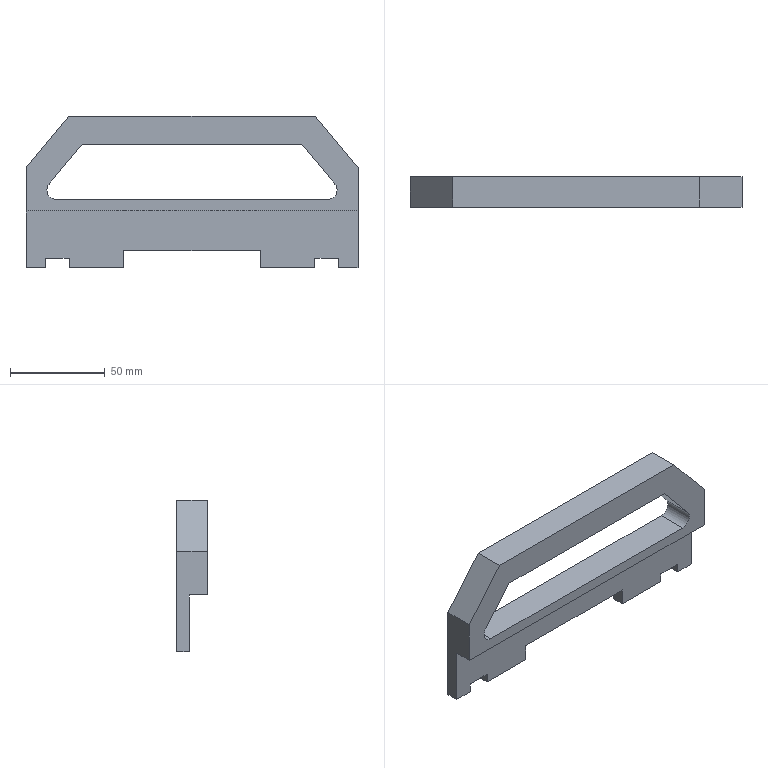Part | STEP file | Computer handle_RR | 1 solid | 38 faces | box 175 x 16 x 80 mm | volume 87445 mm3 | plane 36 | cylinder 2 | commonest cylinder face diameters 10 x2